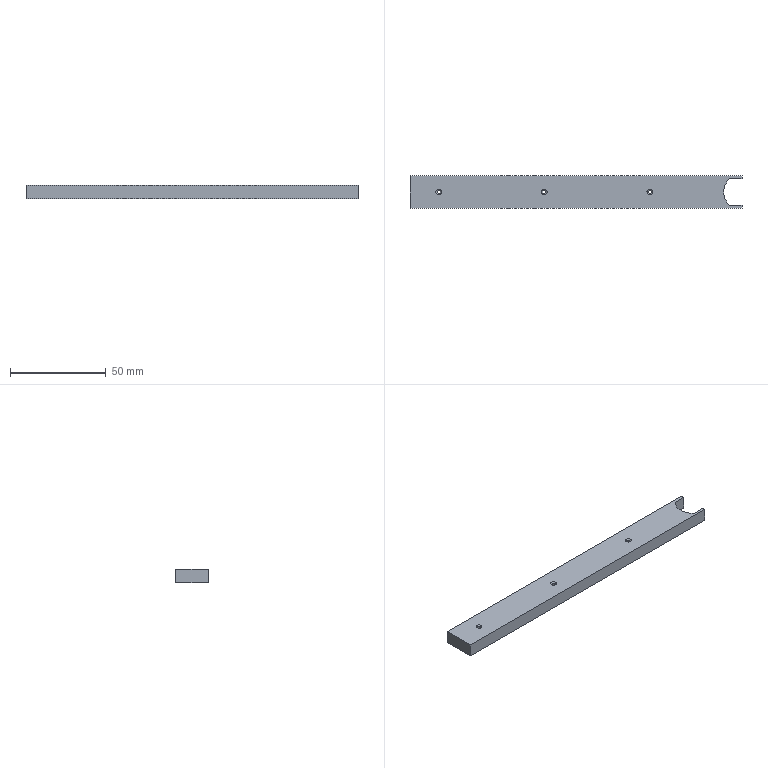Part | STEP file | BU-D02-2b#180 | 1 solid | 22 faces | box 173.003 x 17 x 7 mm | volume 19694 mm3 | plane 9 | cylinder 7 | cone 6 | commonest cylinder face diameters 1.778 x6 18.996 x1